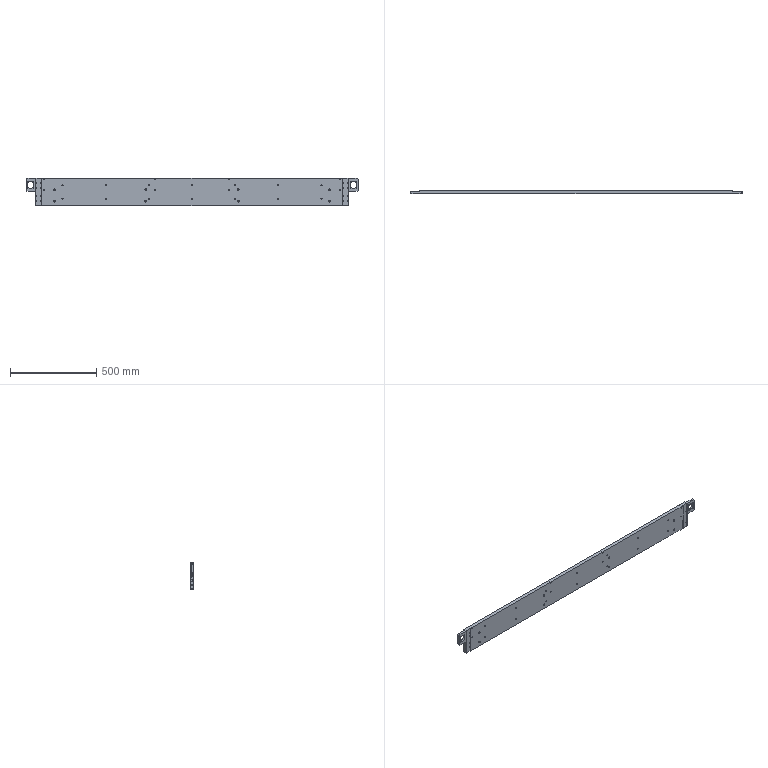Part | SolidWorks | features HoleWzd 9, Cut 4, Chamfer 3, MirrorPattern 3, Fillet 2, Extrusion 1 | 1 solid | 256 faces | box 1924 x 20 x 160 mm | volume 5814736 mm3 | cylinder 186 | plane 50 | cone 20 | commonest cylinder face diameters 4.5 x32 8 x32 6.8 x28 2.5 x20 4.2 x16 5 x16